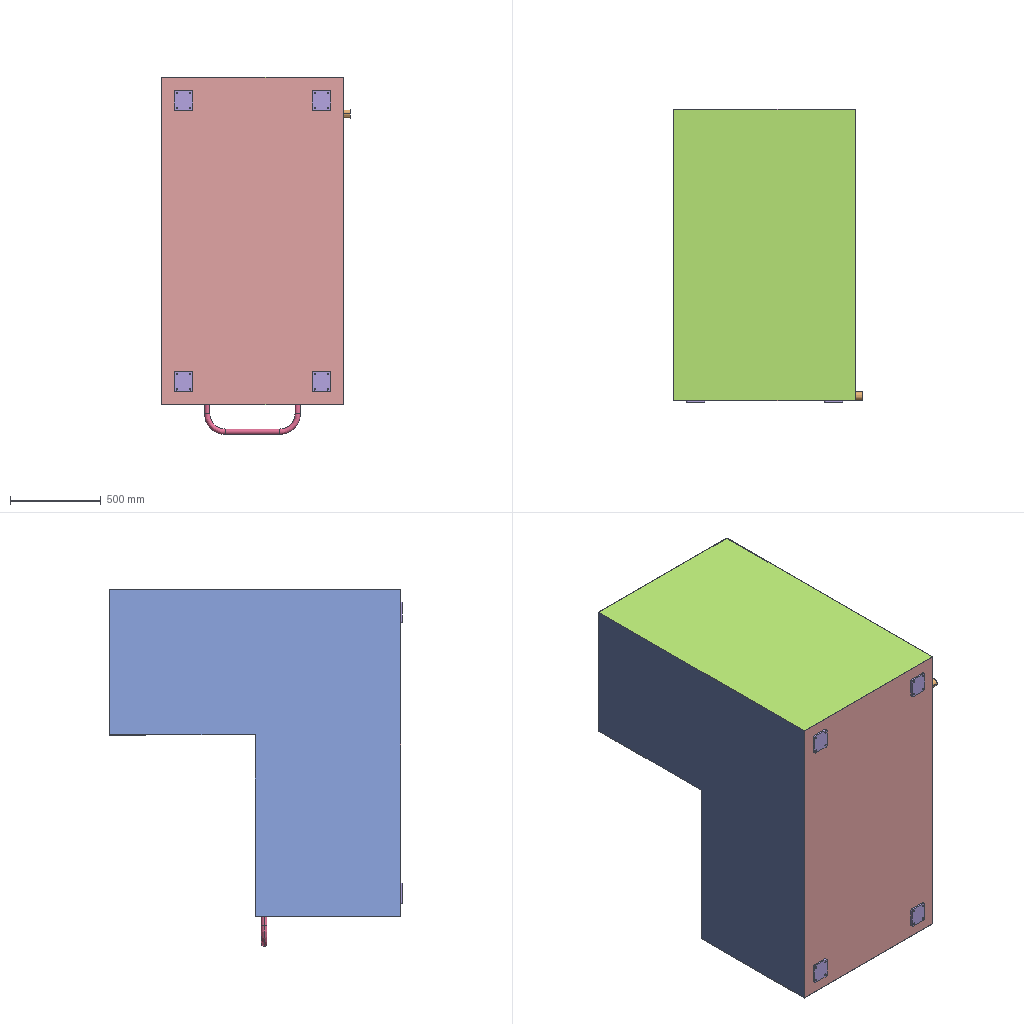Assembly | SolidWorks | 9 different items | 12 placed | box 1039 x 1612 x 1967 mm
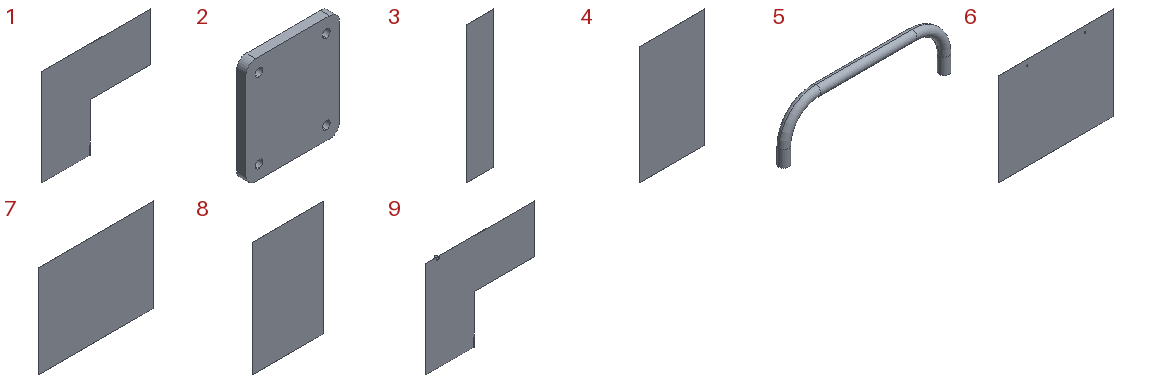Parts list (item | quantity | size | volume | features):
1 | x1 | 1800 x 1 x 1600 mm | 2080000 mm3 | features Extrusion 1
2 | x4 | 100 x 10 x 114 mm | 110872 mm3 | features Extrusion 1, HoleWzd 1
3 | x1 | 200 x 1 x 1000 mm | 200000 mm3 | features Extrusion 1
4 | x1 | 1000 x 1 x 1800 mm | 1800000 mm3 | features Extrusion 1
5 | x1 | 530 x 30 x 165 mm | 501138 mm3 | features HoleWzd 1, Sweep 1
6 | x1 | 1000 x 1 x 801 mm | 800810 mm3 | features Extrusion 1, ICE 1
7 | x1 | 1000 x 1 x 801 mm | 801000 mm3 | features Extrusion 1
8 | x1 | 1000 x 1 x 1601 mm | 1601000 mm3 | features Extrusion 1
9 | x1 | 1800 x 40 x 1600 mm | 2097397 mm3 | features ICE 2, Extrusion 1
Mates (type | each side: item.copy, entity, surface, feature):
Coincident | 4.1 face plane Boss-Extrude1 | 1.1 face plane Boss-Extrude1 | 3 times
Coincident | 8.1 face plane Boss-Extrude1 | 7.1 face plane Boss-Extrude1 | 2 times
Coincident | 7.1 face plane Boss-Extrude1 | 3.1 face plane Boss-Extrude1
Coincident | 7.1 face plane Boss-Extrude1 | 9.1 face plane Boss-Extrude1 | 2 times
Coincident | 8.1 face plane Boss-Extrude1 | 9.1 face plane Boss-Extrude1
Coincident | 4.1 face plane Boss-Extrude1 | 2.1 face plane Boss-Extrude1
Coincident | 2.1 face plane Boss-Extrude1 | 2.2 face plane Boss-Extrude1 | 2 times
Coincident | 2.1 face plane Boss-Extrude1 | 2.3 face plane Boss-Extrude1
Coincident | 2.3 face plane Boss-Extrude1 | 2.4 face plane Boss-Extrude1 | 2 times
Coincident | 2.1 face plane Boss-Extrude1 | 2.4 face plane Boss-Extrude1
Coincident | 2.2 face plane Boss-Extrude1 | 2.3 face plane Boss-Extrude1
DistanceDim | 9.1 face plane Boss-Extrude1 | 2.4 face plane Boss-Extrude1
DistanceDim | 1.1 face plane Boss-Extrude1 | 2.2 face plane Boss-Extrude1
DistanceDim | 8.1 face plane Boss-Extrude1 | 2.2 face plane Boss-Extrude1
Coincident | 9.1 face plane Boss-Extrude1 | 6.1 face plane Boss-Extrude1 | 3 times
Concentric | 6.1 face cylinder Cut-Extrude1 | 5.1 face cylinder Sweep1 | 2 times
Coincident | 6.1 face plane Boss-Extrude1 | 5.1 face plane Sweep1